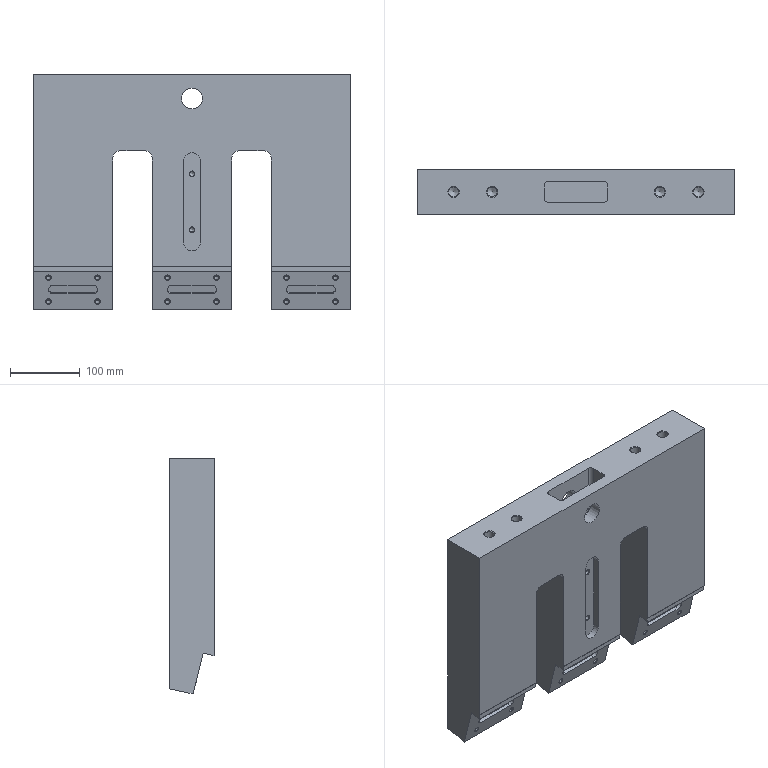Part | NX | features SIMPLE HOLE 20, SYMBOLIC_THREAD 20, DATUM_CSYS 11, SKETCH 10, EXTRUDE 6, HOLE PACKAGE 4, BLEND 1 | 1 solid | 121 faces | box 454 x 65 x 337.24 mm | volume 7495234 mm3 | plane 43 | cone 40 | cylinder 38 | commonest cylinder face diameters 6.8 x16 12 x6 10 x4 14 x4 20 x4 25 x2